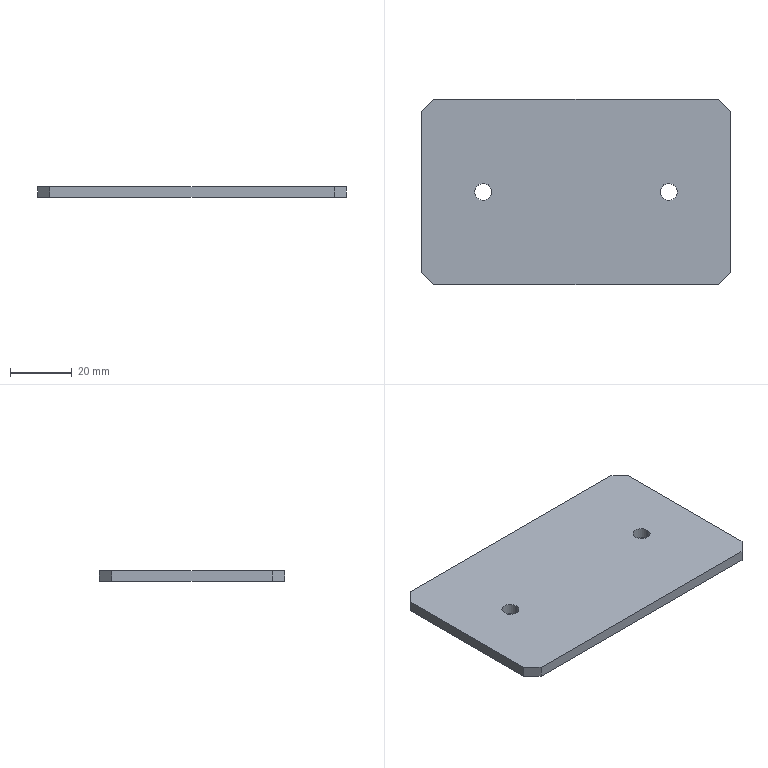Part | STEP file | B1-031 | 1 solid | 14 faces | box 100 x 60 x 3.5 mm | volume 20722 mm3 | plane 10 | cylinder 4 | commonest cylinder face diameters 5.5 x4
STEP:
#1=CARTESIAN_POINT('',(0.,0.,0.));
#2=DIRECTION('',(0.,0.,1.));
#3=DIRECTION('',(1.,0.,0.));
#4=AXIS2_PLACEMENT_3D('',#1,#2,#3);
#5=CARTESIAN_POINT('',(32.75,0.,-1.75));
#6=VERTEX_POINT('',#5);
#7=CARTESIAN_POINT('',(32.75,0.,1.75));
#8=VERTEX_POINT('',#7);
#9=CARTESIAN_POINT('',(32.75,0.,-9.528));
#10=DIRECTION('',(0.,0.,1.));
#11=VECTOR('',#10,1.);
#12=LINE('',#9,#11);
#13=CARTESIAN_POINT('',(30.,0.,-9.528));
#14=DIRECTION('',(0.,0.,1.));
#15=DIRECTION('',(1.,0.,0.));
#16=AXIS2_PLACEMENT_3D('',#13,#14,#15);
#17=CYLINDRICAL_SURFACE('',#16,2.75);
#18=CARTESIAN_POINT('',(6.283,0.));
#19=DIRECTION('',(0.,1.));
#20=VECTOR('',#19,1.);
#21=LINE('',#18,#20);
#22=(GEOMETRIC_REPRESENTATION_CONTEXT(2)PARAMETRIC_REPRESENTATION_CONTEXT()REPRESENTATION_CONTEXT('',''));
#23=DEFINITIONAL_REPRESENTATION('',(#21),#22);
#24=PCURVE('',#17,#23);
#25=CARTESIAN_POINT('',(30.,0.,-9.528));
#26=DIRECTION('',(0.,0.,1.));
#27=DIRECTION('',(1.,0.,0.));
#28=AXIS2_PLACEMENT_3D('',#25,#26,#27);
#29=CYLINDRICAL_SURFACE('',#28,2.75);
#30=CARTESIAN_POINT('',(0.,0.));
#31=DIRECTION('',(0.,1.));
#32=VECTOR('',#31,1.);
#33=LINE('',#30,#32);
#34=(GEOMETRIC_REPRESENTATION_CONTEXT(2)PARAMETRIC_REPRESENTATION_CONTEXT()REPRESENTATION_CONTEXT('',''));
#35=DEFINITIONAL_REPRESENTATION('',(#33),#34);
#36=PCURVE('',#29,#35);
#37=SURFACE_CURVE('',#12,(#24,#36),.PCURVE_S1.);
#38=EDGE_CURVE('',#6,#8,#37,.T.);
#39=ORIENTED_EDGE('',*,*,#38,.T.);
#40=CARTESIAN_POINT('',(27.25,0.,1.75));
#41=VERTEX_POINT('',#40);
#42=CARTESIAN_POINT('',(30.,0.,1.75));
#43=DIRECTION('',(0.,0.,1.));
#44=DIRECTION('',(1.,0.,0.));
#45=AXIS2_PLACEMENT_3D('',#42,#43,#44);
#46=CIRCLE('',#45,2.75);
#47=CARTESIAN_POINT('',(0.,11.278));
#48=DIRECTION('',(1.,0.));
#49=VECTOR('',#48,1.);
#50=LINE('',#47,#49);
#51=(GEOMETRIC_REPRESENTATION_CONTEXT(2)PARAMETRIC_REPRESENTATION_CONTEXT()REPRESENTATION_CONTEXT('',''));
#52=DEFINITIONAL_REPRESENTATION('',(#50),#51);
#53=PCURVE('',#17,#52);
#54=CARTESIAN_POINT('',(0.,0.,1.75));
#55=DIRECTION('',(0.,0.,1.));
#56=DIRECTION('',(1.,0.,0.));
#57=AXIS2_PLACEMENT_3D('',#54,#55,#56);
#58=PLANE('',#57);
#59=CARTESIAN_POINT('',(30.,0.));
#60=DIRECTION('',(1.,0.));
#61=AXIS2_PLACEMENT_2D('',#59,#60);
#62=CIRCLE('',#61,2.75);
#63=(GEOMETRIC_REPRESENTATION_CONTEXT(2)PARAMETRIC_REPRESENTATION_CONTEXT()REPRESENTATION_CONTEXT('',''));
#64=DEFINITIONAL_REPRESENTATION('',(#62),#63);
#65=PCURVE('',#58,#64);
#66=SURFACE_CURVE('',#46,(#53,#65),.PCURVE_S1.);
#67=EDGE_CURVE('',#41,#8,#66,.T.);
#68=ORIENTED_EDGE('',*,*,#67,.F.);
#69=CARTESIAN_POINT('',(27.25,0.,-1.75));
#70=VERTEX_POINT('',#69);
#71=CARTESIAN_POINT('',(27.25,0.,-9.528));
#72=DIRECTION('',(0.,0.,1.));
#73=VECTOR('',#72,1.);
#74=LINE('',#71,#73);
#75=CARTESIAN_POINT('',(3.142,0.));
#76=DIRECTION('',(0.,1.));
#77=VECTOR('',#76,1.);
#78=LINE('',#75,#77);
#79=(GEOMETRIC_REPRESENTATION_CONTEXT(2)PARAMETRIC_REPRESENTATION_CONTEXT()REPRESENTATION_CONTEXT('',''));
#80=DEFINITIONAL_REPRESENTATION('',(#78),#79);
#81=PCURVE('',#17,#80);
#82=CARTESIAN_POINT('',(3.142,0.));
#83=DIRECTION('',(0.,1.));
#84=VECTOR('',#83,1.);
#85=LINE('',#82,#84);
#86=(GEOMETRIC_REPRESENTATION_CONTEXT(2)PARAMETRIC_REPRESENTATION_CONTEXT()REPRESENTATION_CONTEXT('',''));
#87=DEFINITIONAL_REPRESENTATION('',(#85),#86);
#88=PCURVE('',#29,#87);
#89=SURFACE_CURVE('',#74,(#81,#88),.PCURVE_S1.);
#90=EDGE_CURVE('',#70,#41,#89,.T.);
#91=ORIENTED_EDGE('',*,*,#90,.F.);
#92=CARTESIAN_POINT('',(30.,0.,-1.75));
#93=DIRECTION('',(0.,0.,-1.));
#94=DIRECTION('',(1.,0.,0.));
#95=AXIS2_PLACEMENT_3D('',#92,#93,#94);
#96=CIRCLE('',#95,2.75);
#97=CARTESIAN_POINT('',(6.283,7.778));
#98=DIRECTION('',(-1.,0.));
#99=VECTOR('',#98,1.);
#100=LINE('',#97,#99);
#101=(GEOMETRIC_REPRESENTATION_CONTEXT(2)PARAMETRIC_REPRESENTATION_CONTEXT()REPRESENTATION_CONTEXT('',''));
#102=DEFINITIONAL_REPRESENTATION('',(#100),#101);
#103=PCURVE('',#17,#102);
#104=CARTESIAN_POINT('',(0.,0.,-1.75));
#105=DIRECTION('',(0.,0.,1.));
#106=DIRECTION('',(1.,0.,0.));
#107=AXIS2_PLACEMENT_3D('',#104,#105,#106);
#108=PLANE('',#107);
#109=CARTESIAN_POINT('',(32.75,0.));
#110=CARTESIAN_POINT('',(32.75,-4.763));
#111=CARTESIAN_POINT('',(28.625,-2.382));
#112=CARTESIAN_POINT('',(24.5,0.));
#113=CARTESIAN_POINT('',(28.625,2.382));
#114=CARTESIAN_POINT('',(32.75,4.763));
#115=CARTESIAN_POINT('',(32.75,0.));
#116=(BOUNDED_CURVE()B_SPLINE_CURVE(2,(#109,#110,#111,#112,#113,#114,#115),.UNSPECIFIED.,.T.,.F.)B_SPLINE_CURVE_WITH_KNOTS((1,2,2,2,2,1),(-2.094,0.,2.094,4.189,6.283,8.378),.UNSPECIFIED.)CURVE()GEOMETRIC_REPRESENTATION_ITEM()RATIONAL_B_SPLINE_CURVE((1.,0.5,1.,0.5,1.,0.5,1.))REPRESENTATION_ITEM(''));
#117=(GEOMETRIC_REPRESENTATION_CONTEXT(2)PARAMETRIC_REPRESENTATION_CONTEXT()REPRESENTATION_CONTEXT('',''));
#118=DEFINITIONAL_REPRESENTATION('',(#116),#117);
#119=PCURVE('',#108,#118);
#120=SURFACE_CURVE('',#96,(#103,#119),.PCURVE_S1.);
#121=EDGE_CURVE('',#6,#70,#120,.T.);
#122=ORIENTED_EDGE('',*,*,#121,.F.);
#123=EDGE_LOOP('',(#39,#68,#91,#122));
#124=FACE_BOUND('',#123,.F.);
#125=ADVANCED_FACE('',(#124),#17,.F.);
#126=CARTESIAN_POINT('',(-27.25,0.,-1.75));
#127=VERTEX_POINT('',#126);
#128=CARTESIAN_POINT('',(-27.25,0.,1.75));
#129=VERTEX_POINT('',#128);
#130=CARTESIAN_POINT('',(-27.25,0.,-9.528));
#131=DIRECTION('',(0.,0.,1.));
#132=VECTOR('',#131,1.);
#133=LINE('',#130,#132);
#134=CARTESIAN_POINT('',(-30.,0.,-9.528));
#135=DIRECTION('',(0.,0.,1.));
#136=DIRECTION('',(1.,0.,0.));
#137=AXIS2_PLACEMENT_3D('',#134,#135,#136);
#138=CYLINDRICAL_SURFACE('',#137,2.75);
#139=CARTESIAN_POINT('',(6.283,0.));
#140=DIRECTION('',(0.,1.));
#141=VECTOR('',#140,1.);
#142=LINE('',#139,#141);
#143=(GEOMETRIC_REPRESENTATION_CONTEXT(2)PARAMETRIC_REPRESENTATION_CONTEXT()REPRESENTATION_CONTEXT('',''));
#144=DEFINITIONAL_REPRESENTATION('',(#142),#143);
#145=PCURVE('',#138,#144);
#146=CARTESIAN_POINT('',(-30.,0.,-9.528));
#147=DIRECTION('',(0.,0.,1.));
#148=DIRECTION('',(1.,0.,0.));
#149=AXIS2_PLACEMENT_3D('',#146,#147,#148);
#150=CYLINDRICAL_SURFACE('',#149,2.75);
#151=CARTESIAN_POINT('',(0.,0.));
#152=DIRECTION('',(0.,1.));
#153=VECTOR('',#152,1.);
#154=LINE('',#151,#153);
#155=(GEOMETRIC_REPRESENTATION_CONTEXT(2)PARAMETRIC_REPRESENTATION_CONTEXT()REPRESENTATION_CONTEXT('',''));
#156=DEFINITIONAL_REPRESENTATION('',(#154),#155);
#157=PCURVE('',#150,#156);
#158=SURFACE_CURVE('',#133,(#145,#157),.PCURVE_S1.);
#159=EDGE_CURVE('',#127,#129,#158,.T.);
#160=ORIENTED_EDGE('',*,*,#159,.T.);
#161=CARTESIAN_POINT('',(-32.75,0.,1.75));
#162=VERTEX_POINT('',#161);
#163=CARTESIAN_POINT('',(-30.,0.,1.75));
#164=DIRECTION('',(0.,0.,1.));
#165=DIRECTION('',(1.,0.,0.));
#166=AXIS2_PLACEMENT_3D('',#163,#164,#165);
#167=CIRCLE('',#166,2.75);
#168=CARTESIAN_POINT('',(0.,11.278));
#169=DIRECTION('',(1.,0.));
#170=VECTOR('',#169,1.);
#171=LINE('',#168,#170);
#172=(GEOMETRIC_REPRESENTATION_CONTEXT(2)PARAMETRIC_REPRESENTATION_CONTEXT()REPRESENTATION_CONTEXT('',''));
#173=DEFINITIONAL_REPRESENTATION('',(#171),#172);
#174=PCURVE('',#138,#173);
#175=CARTESIAN_POINT('',(-30.,0.));
#176=DIRECTION('',(1.,0.));
#177=AXIS2_PLACEMENT_2D('',#175,#176);
#178=CIRCLE('',#177,2.75);
#179=(GEOMETRIC_REPRESENTATION_CONTEXT(2)PARAMETRIC_REPRESENTATION_CONTEXT()REPRESENTATION_CONTEXT('',''));
#180=DEFINITIONAL_REPRESENTATION('',(#178),#179);
#181=PCURVE('',#58,#180);
#182=SURFACE_CURVE('',#167,(#174,#181),.PCURVE_S1.);
#183=EDGE_CURVE('',#162,#129,#182,.T.);
#184=ORIENTED_EDGE('',*,*,#183,.F.);
#185=CARTESIAN_POINT('',(-32.75,0.,-1.75));
#186=VERTEX_POINT('',#185);
#187=CARTESIAN_POINT('',(-32.75,0.,-9.528));
#188=DIRECTION('',(0.,0.,1.));
#189=VECTOR('',#188,1.);
#190=LINE('',#187,#189);
#191=CARTESIAN_POINT('',(3.142,0.));
#192=DIRECTION('',(0.,1.));
#193=VECTOR('',#192,1.);
#194=LINE('',#191,#193);
#195=(GEOMETRIC_REPRESENTATION_CONTEXT(2)PARAMETRIC_REPRESENTATION_CONTEXT()REPRESENTATION_CONTEXT('',''));
#196=DEFINITIONAL_REPRESENTATION('',(#194),#195);
#197=PCURVE('',#138,#196);
#198=CARTESIAN_POINT('',(3.142,0.));
#199=DIRECTION('',(0.,1.));
#200=VECTOR('',#199,1.);
#201=LINE('',#198,#200);
#202=(GEOMETRIC_REPRESENTATION_CONTEXT(2)PARAMETRIC_REPRESENTATION_CONTEXT()REPRESENTATION_CONTEXT('',''));
#203=DEFINITIONAL_REPRESENTATION('',(#201),#202);
#204=PCURVE('',#150,#203);
#205=SURFACE_CURVE('',#190,(#197,#204),.PCURVE_S1.);
#206=EDGE_CURVE('',#186,#162,#205,.T.);
#207=ORIENTED_EDGE('',*,*,#206,.F.);
#208=CARTESIAN_POINT('',(-30.,0.,-1.75));
#209=DIRECTION('',(0.,0.,-1.));
#210=DIRECTION('',(1.,0.,0.));
#211=AXIS2_PLACEMENT_3D('',#208,#209,#210);
#212=CIRCLE('',#211,2.75);
#213=CARTESIAN_POINT('',(6.283,7.778));
#214=DIRECTION('',(-1.,0.));
#215=VECTOR('',#214,1.);
#216=LINE('',#213,#215);
#217=(GEOMETRIC_REPRESENTATION_CONTEXT(2)PARAMETRIC_REPRESENTATION_CONTEXT()REPRESENTATION_CONTEXT('',''));
#218=DEFINITIONAL_REPRESENTATION('',(#216),#217);
#219=PCURVE('',#138,#218);
#220=CARTESIAN_POINT('',(-27.25,0.));
#221=CARTESIAN_POINT('',(-27.25,-4.763));
#222=CARTESIAN_POINT('',(-31.375,-2.382));
#223=CARTESIAN_POINT('',(-35.5,0.));
#224=CARTESIAN_POINT('',(-31.375,2.382));
#225=CARTESIAN_POINT('',(-27.25,4.763));
#226=CARTESIAN_POINT('',(-27.25,0.));
#227=(BOUNDED_CURVE()B_SPLINE_CURVE(2,(#220,#221,#222,#223,#224,#225,#226),.UNSPECIFIED.,.T.,.F.)B_SPLINE_CURVE_WITH_KNOTS((1,2,2,2,2,1),(-2.094,0.,2.094,4.189,6.283,8.378),.UNSPECIFIED.)CURVE()GEOMETRIC_REPRESENTATION_ITEM()RATIONAL_B_SPLINE_CURVE((1.,0.5,1.,0.5,1.,0.5,1.))REPRESENTATION_ITEM(''));
#228=(GEOMETRIC_REPRESENTATION_CONTEXT(2)PARAMETRIC_REPRESENTATION_CONTEXT()REPRESENTATION_CONTEXT('',''));
#229=DEFINITIONAL_REPRESENTATION('',(#227),#228);
#230=PCURVE('',#108,#229);
#231=SURFACE_CURVE('',#212,(#219,#230),.PCURVE_S1.);
#232=EDGE_CURVE('',#127,#186,#231,.T.);
#233=ORIENTED_EDGE('',*,*,#232,.F.);
#234=EDGE_LOOP('',(#160,#184,#207,#233));
#235=FACE_BOUND('',#234,.F.);
#236=ADVANCED_FACE('',(#235),#138,.F.);
#237=CARTESIAN_POINT('',(50.,-26.,1.75));
#238=VERTEX_POINT('',#237);
#239=CARTESIAN_POINT('',(50.,26.,1.75));
#240=VERTEX_POINT('',#239);
#241=CARTESIAN_POINT('',(50.,30.,1.75));
#242=DIRECTION('',(0.,1.,0.));
#243=VECTOR('',#242,1.);
#244=LINE('',#241,#243);
#245=CARTESIAN_POINT('',(50.,30.,1.75));
#246=DIRECTION('',(-1.,0.,0.));
#247=DIRECTION('',(0.,0.,1.));
#248=AXIS2_PLACEMENT_3D('',#245,#246,#247);
#249=PLANE('',#248);
#250=CARTESIAN_POINT('',(0.,0.));
#251=DIRECTION('',(0.,1.));
#252=VECTOR('',#251,1.);
#253=LINE('',#250,#252);
#254=(GEOMETRIC_REPRESENTATION_CONTEXT(2)PARAMETRIC_REPRESENTATION_CONTEXT()REPRESENTATION_CONTEXT('',''));
#255=DEFINITIONAL_REPRESENTATION('',(#253),#254);
#256=PCURVE('',#249,#255);
#257=CARTESIAN_POINT('',(50.,30.));
#258=DIRECTION('',(0.,1.));
#259=VECTOR('',#258,1.);
#260=LINE('',#257,#259);
#261=(GEOMETRIC_REPRESENTATION_CONTEXT(2)PARAMETRIC_REPRESENTATION_CONTEXT()REPRESENTATION_CONTEXT('',''));
#262=DEFINITIONAL_REPRESENTATION('',(#260),#261);
#263=PCURVE('',#58,#262);
#264=SURFACE_CURVE('',#244,(#256,#263),.PCURVE_S1.);
#265=EDGE_CURVE('',#238,#240,#264,.T.);
#266=ORIENTED_EDGE('',*,*,#265,.F.);
#267=CARTESIAN_POINT('',(50.,-26.,-1.75));
#268=VERTEX_POINT('',#267);
#269=CARTESIAN_POINT('',(50.,-26.,1.75));
#270=DIRECTION('',(0.,0.,-1.));
#271=VECTOR('',#270,1.);
#272=LINE('',#269,#271);
#273=CARTESIAN_POINT('',(0.,-56.));
#274=DIRECTION('',(-1.,0.));
#275=VECTOR('',#274,1.);
#276=LINE('',#273,#275);
#277=(GEOMETRIC_REPRESENTATION_CONTEXT(2)PARAMETRIC_REPRESENTATION_CONTEXT()REPRESENTATION_CONTEXT('',''));
#278=DEFINITIONAL_REPRESENTATION('',(#276),#277);
#279=PCURVE('',#249,#278);
#280=CARTESIAN_POINT('',(50.,-26.,1.75));
#281=DIRECTION('',(-0.7071,0.7071,0.));
#282=DIRECTION('',(0.,0.,-1.));
#283=AXIS2_PLACEMENT_3D('',#280,#281,#282);
#284=PLANE('',#283);
#285=CARTESIAN_POINT('',(0.,0.));
#286=DIRECTION('',(1.,0.));
#287=VECTOR('',#286,1.);
#288=LINE('',#285,#287);
#289=(GEOMETRIC_REPRESENTATION_CONTEXT(2)PARAMETRIC_REPRESENTATION_CONTEXT()REPRESENTATION_CONTEXT('',''));
#290=DEFINITIONAL_REPRESENTATION('',(#288),#289);
#291=PCURVE('',#284,#290);
#292=SURFACE_CURVE('',#272,(#279,#291),.PCURVE_S1.);
#293=EDGE_CURVE('',#238,#268,#292,.T.);
#294=ORIENTED_EDGE('',*,*,#293,.T.);
#295=CARTESIAN_POINT('',(50.,26.,-1.75));
#296=VERTEX_POINT('',#295);
#297=CARTESIAN_POINT('',(50.,30.,-1.75));
#298=DIRECTION('',(0.,1.,0.));
#299=VECTOR('',#298,1.);
#300=LINE('',#297,#299);
#301=CARTESIAN_POINT('',(-3.5,0.));
#302=DIRECTION('',(0.,1.));
#303=VECTOR('',#302,1.);
#304=LINE('',#301,#303);
#305=(GEOMETRIC_REPRESENTATION_CONTEXT(2)PARAMETRIC_REPRESENTATION_CONTEXT()REPRESENTATION_CONTEXT('',''));
#306=DEFINITIONAL_REPRESENTATION('',(#304),#305);
#307=PCURVE('',#249,#306);
#308=CARTESIAN_POINT('',(50.,30.));
#309=DIRECTION('',(0.,1.));
#310=VECTOR('',#309,1.);
#311=LINE('',#308,#310);
#312=(GEOMETRIC_REPRESENTATION_CONTEXT(2)PARAMETRIC_REPRESENTATION_CONTEXT()REPRESENTATION_CONTEXT('',''));
#313=DEFINITIONAL_REPRESENTATION('',(#311),#312);
#314=PCURVE('',#108,#313);
#315=SURFACE_CURVE('',#300,(#307,#314),.PCURVE_S1.);
#316=EDGE_CURVE('',#268,#296,#315,.T.);
#317=ORIENTED_EDGE('',*,*,#316,.T.);
#318=CARTESIAN_POINT('',(50.,26.,1.75));
#319=DIRECTION('',(0.,0.,1.));
#320=VECTOR('',#319,1.);
#321=LINE('',#318,#320);
#322=CARTESIAN_POINT('',(0.,-4.));
#323=DIRECTION('',(1.,0.));
#324=VECTOR('',#323,1.);
#325=LINE('',#322,#324);
#326=(GEOMETRIC_REPRESENTATION_CONTEXT(2)PARAMETRIC_REPRESENTATION_CONTEXT()REPRESENTATION_CONTEXT('',''));
#327=DEFINITIONAL_REPRESENTATION('',(#325),#326);
#328=PCURVE('',#249,#327);
#329=CARTESIAN_POINT('',(46.,30.,1.75));
#330=DIRECTION('',(-0.7071,-0.7071,0.));
#331=DIRECTION('',(0.,0.,-1.));
#332=AXIS2_PLACEMENT_3D('',#329,#330,#331);
#333=PLANE('',#332);
#334=CARTESIAN_POINT('',(0.,5.657));
#335=DIRECTION('',(-1.,0.));
#336=VECTOR('',#335,1.);
#337=LINE('',#334,#336);
#338=(GEOMETRIC_REPRESENTATION_CONTEXT(2)PARAMETRIC_REPRESENTATION_CONTEXT()REPRESENTATION_CONTEXT('',''));
#339=DEFINITIONAL_REPRESENTATION('',(#337),#338);
#340=PCURVE('',#333,#339);
#341=SURFACE_CURVE('',#321,(#328,#340),.PCURVE_S1.);
#342=EDGE_CURVE('',#296,#240,#341,.T.);
#343=ORIENTED_EDGE('',*,*,#342,.T.);
#344=EDGE_LOOP('',(#266,#294,#317,#343));
#345=FACE_BOUND('',#344,.T.);
#346=ADVANCED_FACE('',(#345),#249,.F.);
#347=CARTESIAN_POINT('',(46.,30.,-1.75));
#348=VERTEX_POINT('',#347);
#349=CARTESIAN_POINT('',(-46.,30.,-1.75));
#350=VERTEX_POINT('',#349);
#351=CARTESIAN_POINT('',(-50.,30.,-1.75));
#352=DIRECTION('',(-1.,0.,0.));
#353=VECTOR('',#352,1.);
#354=LINE('',#351,#353);
#355=CARTESIAN_POINT('',(-50.,30.,1.75));
#356=DIRECTION('',(0.,-1.,0.));
#357=DIRECTION('',(0.,0.,-1.));
#358=AXIS2_PLACEMENT_3D('',#355,#356,#357);
#359=PLANE('',#358);
#360=CARTESIAN_POINT('',(3.5,0.));
#361=DIRECTION('',(0.,-1.));
#362=VECTOR('',#361,1.);
#363=LINE('',#360,#362);
#364=(GEOMETRIC_REPRESENTATION_CONTEXT(2)PARAMETRIC_REPRESENTATION_CONTEXT()REPRESENTATION_CONTEXT('',''));
#365=DEFINITIONAL_REPRESENTATION('',(#363),#364);
#366=PCURVE('',#359,#365);
#367=CARTESIAN_POINT('',(-50.,30.));
#368=DIRECTION('',(-1.,0.));
#369=VECTOR('',#368,1.);
#370=LINE('',#367,#369);
#371=(GEOMETRIC_REPRESENTATION_CONTEXT(2)PARAMETRIC_REPRESENTATION_CONTEXT()REPRESENTATION_CONTEXT('',''));
#372=DEFINITIONAL_REPRESENTATION('',(#370),#371);
#373=PCURVE('',#108,#372);
#374=SURFACE_CURVE('',#354,(#366,#373),.PCURVE_S1.);
#375=EDGE_CURVE('',#348,#350,#374,.T.);
#376=ORIENTED_EDGE('',*,*,#375,.T.);
#377=CARTESIAN_POINT('',(-46.,30.,1.75));
#378=VERTEX_POINT('',#377);
#379=CARTESIAN_POINT('',(-46.,30.,1.75));
#380=DIRECTION('',(0.,0.,1.));
#381=VECTOR('',#380,1.);
#382=LINE('',#379,#381);
#383=CARTESIAN_POINT('',(0.,4.));
#384=DIRECTION('',(-1.,0.));
#385=VECTOR('',#384,1.);
#386=LINE('',#383,#385);
#387=(GEOMETRIC_REPRESENTATION_CONTEXT(2)PARAMETRIC_REPRESENTATION_CONTEXT()REPRESENTATION_CONTEXT('',''));
#388=DEFINITIONAL_REPRESENTATION('',(#386),#387);
#389=PCURVE('',#359,#388);
#390=CARTESIAN_POINT('',(-50.,26.,1.75));
#391=DIRECTION('',(0.7071,-0.7071,0.));
#392=DIRECTION('',(0.,0.,-1.));
#393=AXIS2_PLACEMENT_3D('',#390,#391,#392);
#394=PLANE('',#393);
#395=CARTESIAN_POINT('',(0.,5.657));
#396=DIRECTION('',(-1.,0.));
#397=VECTOR('',#396,1.);
#398=LINE('',#395,#397);
#399=(GEOMETRIC_REPRESENTATION_CONTEXT(2)PARAMETRIC_REPRESENTATION_CONTEXT()REPRESENTATION_CONTEXT('',''));
#400=DEFINITIONAL_REPRESENTATION('',(#398),#399);
#401=PCURVE('',#394,#400);
#402=SURFACE_CURVE('',#382,(#389,#401),.PCURVE_S1.);
#403=EDGE_CURVE('',#350,#378,#402,.T.);
#404=ORIENTED_EDGE('',*,*,#403,.T.);
#405=CARTESIAN_POINT('',(46.,30.,1.75));
#406=VERTEX_POINT('',#405);
#407=CARTESIAN_POINT('',(-50.,30.,1.75));
#408=DIRECTION('',(-1.,0.,0.));
#409=VECTOR('',#408,1.);
#410=LINE('',#407,#409);
#411=CARTESIAN_POINT('',(0.,0.));
#412=DIRECTION('',(0.,-1.));
#413=VECTOR('',#412,1.);
#414=LINE('',#411,#413);
#415=(GEOMETRIC_REPRESENTATION_CONTEXT(2)PARAMETRIC_REPRESENTATION_CONTEXT()REPRESENTATION_CONTEXT('',''));
#416=DEFINITIONAL_REPRESENTATION('',(#414),#415);
#417=PCURVE('',#359,#416);
#418=CARTESIAN_POINT('',(-50.,30.));
#419=DIRECTION('',(-1.,0.));
#420=VECTOR('',#419,1.);
#421=LINE('',#418,#420);
#422=(GEOMETRIC_REPRESENTATION_CONTEXT(2)PARAMETRIC_REPRESENTATION_CONTEXT()REPRESENTATION_CONTEXT('',''));
#423=DEFINITIONAL_REPRESENTATION('',(#421),#422);
#424=PCURVE('',#58,#423);
#425=SURFACE_CURVE('',#410,(#417,#424),.PCURVE_S1.);
#426=EDGE_CURVE('',#406,#378,#425,.T.);
#427=ORIENTED_EDGE('',*,*,#426,.F.);
#428=CARTESIAN_POINT('',(46.,30.,1.75));
#429=DIRECTION('',(0.,0.,-1.));
#430=VECTOR('',#429,1.);
#431=LINE('',#428,#430);
#432=CARTESIAN_POINT('',(0.,96.));
#433=DIRECTION('',(1.,0.));
#434=VECTOR('',#433,1.);
#435=LINE('',#432,#434);
#436=(GEOMETRIC_REPRESENTATION_CONTEXT(2)PARAMETRIC_REPRESENTATION_CONTEXT()REPRESENTATION_CONTEXT('',''));
#437=DEFINITIONAL_REPRESENTATION('',(#435),#436);
#438=PCURVE('',#359,#437);
#439=CARTESIAN_POINT('',(0.,0.));
#440=DIRECTION('',(1.,0.));
#441=VECTOR('',#440,1.);
#442=LINE('',#439,#441);
#443=(GEOMETRIC_REPRESENTATION_CONTEXT(2)PARAMETRIC_REPRESENTATION_CONTEXT()REPRESENTATION_CONTEXT('',''));
#444=DEFINITIONAL_REPRESENTATION('',(#442),#443);
#445=PCURVE('',#333,#444);
#446=SURFACE_CURVE('',#431,(#438,#445),.PCURVE_S1.);
#447=EDGE_CURVE('',#406,#348,#446,.T.);
#448=ORIENTED_EDGE('',*,*,#447,.T.);
#449=EDGE_LOOP('',(#376,#404,#427,#448));
#450=FACE_BOUND('',#449,.T.);
#451=ADVANCED_FACE('',(#450),#359,.F.);
#452=CARTESIAN_POINT('',(-50.,26.,1.75));
#453=VERTEX_POINT('',#452);
#454=CARTESIAN_POINT('',(-50.,-26.,1.75));
#455=VERTEX_POINT('',#454);
#456=CARTESIAN_POINT('',(-50.,30.,1.75));
#457=DIRECTION('',(0.,-1.,0.));
#458=VECTOR('',#457,1.);
#459=LINE('',#456,#458);
#460=CARTESIAN_POINT('',(-50.,30.,1.75));
#461=DIRECTION('',(1.,0.,0.));
#462=DIRECTION('',(0.,0.,-1.));
#463=AXIS2_PLACEMENT_3D('',#460,#461,#462);
#464=PLANE('',#463);
#465=CARTESIAN_POINT('',(0.,0.));
#466=DIRECTION('',(0.,-1.));
#467=VECTOR('',#466,1.);
#468=LINE('',#465,#467);
#469=(GEOMETRIC_REPRESENTATION_CONTEXT(2)PARAMETRIC_REPRESENTATION_CONTEXT()REPRESENTATION_CONTEXT('',''));
#470=DEFINITIONAL_REPRESENTATION('',(#468),#469);
#471=PCURVE('',#464,#470);
#472=CARTESIAN_POINT('',(-50.,30.));
#473=DIRECTION('',(0.,-1.));
#474=VECTOR('',#473,1.);
#475=LINE('',#472,#474);
#476=(GEOMETRIC_REPRESENTATION_CONTEXT(2)PARAMETRIC_REPRESENTATION_CONTEXT()REPRESENTATION_CONTEXT('',''));
#477=DEFINITIONAL_REPRESENTATION('',(#475),#476);
#478=PCURVE('',#58,#477);
#479=SURFACE_CURVE('',#459,(#471,#478),.PCURVE_S1.);
#480=EDGE_CURVE('',#453,#455,#479,.T.);
#481=ORIENTED_EDGE('',*,*,#480,.F.);
#482=CARTESIAN_POINT('',(-50.,26.,-1.75));
#483=VERTEX_POINT('',#482);
#484=CARTESIAN_POINT('',(-50.,26.,1.75));
#485=DIRECTION('',(0.,0.,-1.));
#486=VECTOR('',#485,1.);
#487=LINE('',#484,#486);
#488=CARTESIAN_POINT('',(0.,-4.));
#489=DIRECTION('',(1.,0.));
#490=VECTOR('',#489,1.);
#491=LINE('',#488,#490);
#492=(GEOMETRIC_REPRESENTATION_CONTEXT(2)PARAMETRIC_REPRESENTATION_CONTEXT()REPRESENTATION_CONTEXT('',''));
#493=DEFINITIONAL_REPRESENTATION('',(#491),#492);
#494=PCURVE('',#464,#493);
#495=CARTESIAN_POINT('',(0.,0.));
#496=DIRECTION('',(1.,0.));
#497=VECTOR('',#496,1.);
#498=LINE('',#495,#497);
#499=(GEOMETRIC_REPRESENTATION_CONTEXT(2)PARAMETRIC_REPRESENTATION_CONTEXT()REPRESENTATION_CONTEXT('',''));
#500=DEFINITIONAL_REPRESENTATION('',(#498),#499);
#501=PCURVE('',#394,#500);
#502=SURFACE_CURVE('',#487,(#494,#501),.PCURVE_S1.);
#503=EDGE_CURVE('',#453,#483,#502,.T.);
#504=ORIENTED_EDGE('',*,*,#503,.T.);
#505=CARTESIAN_POINT('',(-50.,-26.,-1.75));
#506=VERTEX_POINT('',#505);
#507=CARTESIAN_POINT('',(-50.,30.,-1.75));
#508=DIRECTION('',(0.,-1.,0.));
#509=VECTOR('',#508,1.);
#510=LINE('',#507,#509);
#511=CARTESIAN_POINT('',(3.5,0.));
#512=DIRECTION('',(0.,-1.));
#513=VECTOR('',#512,1.);
#514=LINE('',#511,#513);
#515=(GEOMETRIC_REPRESENTATION_CONTEXT(2)PARAMETRIC_REPRESENTATION_CONTEXT()REPRESENTATION_CONTEXT('',''));
#516=DEFINITIONAL_REPRESENTATION('',(#514),#515);
#517=PCURVE('',#464,#516);
#518=CARTESIAN_POINT('',(-50.,30.));
#519=DIRECTION('',(0.,-1.));
#520=VECTOR('',#519,1.);
#521=LINE('',#518,#520);
#522=(GEOMETRIC_REPRESENTATION_CONTEXT(2)PARAMETRIC_REPRESENTATION_CONTEXT()REPRESENTATION_CONTEXT('',''));
#523=DEFINITIONAL_REPRESENTATION('',(#521),#522);
#524=PCURVE('',#108,#523);
#525=SURFACE_CURVE('',#510,(#517,#524),.PCURVE_S1.);
#526=EDGE_CURVE('',#483,#506,#525,.T.);
#527=ORIENTED_EDGE('',*,*,#526,.T.);
#528=CARTESIAN_POINT('',(-50.,-26.,1.75));
#529=DIRECTION('',(0.,0.,1.));
#530=VECTOR('',#529,1.);
#531=LINE('',#528,#530);
#532=CARTESIAN_POINT('',(0.,-56.));
#533=DIRECTION('',(-1.,0.));
#534=VECTOR('',#533,1.);
#535=LINE('',#532,#534);
#536=(GEOMETRIC_REPRESENTATION_CONTEXT(2)PARAMETRIC_REPRESENTATION_CONTEXT()REPRESENTATION_CONTEXT('',''));
#537=DEFINITIONAL_REPRESENTATION('',(#535),#536);
#538=PCURVE('',#464,#537);
#539=CARTESIAN_POINT('',(-46.,-30.,1.75));
#540=DIRECTION('',(0.7071,0.7071,0.));
#541=DIRECTION('',(0.,0.,-1.));
#542=AXIS2_PLACEMENT_3D('',#539,#540,#541);
#543=PLANE('',#542);
#544=CARTESIAN_POINT('',(0.,5.657));
#545=DIRECTION('',(-1.,0.));
#546=VECTOR('',#545,1.);
#547=LINE('',#544,#546);
#548=(GEOMETRIC_REPRESENTATION_CONTEXT(2)PARAMETRIC_REPRESENTATION_CONTEXT()REPRESENTATION_CONTEXT('',''));
#549=DEFINITIONAL_REPRESENTATION('',(#547),#548);
#550=PCURVE('',#543,#549);
#551=SURFACE_CURVE('',#531,(#538,#550),.PCURVE_S1.);
#552=EDGE_CURVE('',#506,#455,#551,.T.);
#553=ORIENTED_EDGE('',*,*,#552,.T.);
#554=EDGE_LOOP('',(#481,#504,#527,#553));
#555=FACE_BOUND('',#554,.T.);
#556=ADVANCED_FACE('',(#555),#464,.F.);
#557=CARTESIAN_POINT('',(-46.,-30.,1.75));
#558=VERTEX_POINT('',#557);
#559=CARTESIAN_POINT('',(46.,-30.,1.75));
#560=VERTEX_POINT('',#559);
#561=CARTESIAN_POINT('',(-50.,-30.,1.75));
#562=DIRECTION('',(1.,0.,0.));
#563=VECTOR('',#562,1.);
#564=LINE('',#561,#563);
#565=CARTESIAN_POINT('',(-50.,-30.,1.75));
#566=DIRECTION('',(0.,1.,0.));
#567=DIRECTION('',(0.,0.,1.));
#568=AXIS2_PLACEMENT_3D('',#565,#566,#567);
#569=PLANE('',#568);
#570=CARTESIAN_POINT('',(0.,0.));
#571=DIRECTION('',(0.,1.));
#572=VECTOR('',#571,1.);
#573=LINE('',#570,#572);
#574=(GEOMETRIC_REPRESENTATION_CONTEXT(2)PARAMETRIC_REPRESENTATION_CONTEXT()REPRESENTATION_CONTEXT('',''));
#575=DEFINITIONAL_REPRESENTATION('',(#573),#574);
#576=PCURVE('',#569,#575);
#577=CARTESIAN_POINT('',(-50.,-30.));
#578=DIRECTION('',(1.,0.));
#579=VECTOR('',#578,1.);
#580=LINE('',#577,#579);
#581=(GEOMETRIC_REPRESENTATION_CONTEXT(2)PARAMETRIC_REPRESENTATION_CONTEXT()REPRESENTATION_CONTEXT('',''));
#582=DEFINITIONAL_REPRESENTATION('',(#580),#581);
#583=PCURVE('',#58,#582);
#584=SURFACE_CURVE('',#564,(#576,#583),.PCURVE_S1.);
#585=EDGE_CURVE('',#558,#560,#584,.T.);
#586=ORIENTED_EDGE('',*,*,#585,.F.);
#587=CARTESIAN_POINT('',(-46.,-30.,-1.75));
#588=VERTEX_POINT('',#587);
#589=CARTESIAN_POINT('',(-46.,-30.,1.75));
#590=DIRECTION('',(0.,0.,-1.));
#591=VECTOR('',#590,1.);
#592=LINE('',#589,#591);
#593=CARTESIAN_POINT('',(0.,4.));
#594=DIRECTION('',(-1.,0.));
#595=VECTOR('',#594,1.);
#596=LINE('',#593,#595);
#597=(GEOMETRIC_REPRESENTATION_CONTEXT(2)PARAMETRIC_REPRESENTATION_CONTEXT()REPRESENTATION_CONTEXT('',''));
#598=DEFINITIONAL_REPRESENTATION('',(#596),#597);
#599=PCURVE('',#569,#598);
#600=CARTESIAN_POINT('',(0.,0.));
#601=DIRECTION('',(1.,0.));
#602=VECTOR('',#601,1.);
#603=LINE('',#600,#602);
#604=(GEOMETRIC_REPRESENTATION_CONTEXT(2)PARAMETRIC_REPRESENTATION_CONTEXT()REPRESENTATION_CONTEXT('',''));
#605=DEFINITIONAL_REPRESENTATION('',(#603),#604);
#606=PCURVE('',#543,#605);
#607=SURFACE_CURVE('',#592,(#599,#606),.PCURVE_S1.);
#608=EDGE_CURVE('',#558,#588,#607,.T.);
#609=ORIENTED_EDGE('',*,*,#608,.T.);
#610=CARTESIAN_POINT('',(46.,-30.,-1.75));
#611=VERTEX_POINT('',#610);
#612=CARTESIAN_POINT('',(-50.,-30.,-1.75));
#613=DIRECTION('',(1.,0.,0.));
#614=VECTOR('',#613,1.);
#615=LINE('',#612,#614);
#616=CARTESIAN_POINT('',(-3.5,0.));
#617=DIRECTION('',(0.,1.));
#618=VECTOR('',#617,1.);
#619=LINE('',#616,#618);
#620=(GEOMETRIC_REPRESENTATION_CONTEXT(2)PARAMETRIC_REPRESENTATION_CONTEXT()REPRESENTATION_CONTEXT('',''));
#621=DEFINITIONAL_REPRESENTATION('',(#619),#620);
#622=PCURVE('',#569,#621);
#623=CARTESIAN_POINT('',(-50.,-30.));
#624=DIRECTION('',(1.,0.));
#625=VECTOR('',#624,1.);
#626=LINE('',#623,#625);
#627=(GEOMETRIC_REPRESENTATION_CONTEXT(2)PARAMETRIC_REPRESENTATION_CONTEXT()REPRESENTATION_CONTEXT('',''));
#628=DEFINITIONAL_REPRESENTATION('',(#626),#627);
#629=PCURVE('',#108,#628);
#630=SURFACE_CURVE('',#615,(#622,#629),.PCURVE_S1.);
#631=EDGE_CURVE('',#588,#611,#630,.T.);
#632=ORIENTED_EDGE('',*,*,#631,.T.);
#633=CARTESIAN_POINT('',(46.,-30.,1.75));
#634=DIRECTION('',(0.,0.,1.));
#635=VECTOR('',#634,1.);
#636=LINE('',#633,#635);
#637=CARTESIAN_POINT('',(0.,96.));
#638=DIRECTION('',(1.,0.));
#639=VECTOR('',#638,1.);
#640=LINE('',#637,#639);
#641=(GEOMETRIC_REPRESENTATION_CONTEXT(2)PARAMETRIC_REPRESENTATION_CONTEXT()REPRESENTATION_CONTEXT('',''));
#642=DEFINITIONAL_REPRESENTATION('',(#640),#641);
#643=PCURVE('',#569,#642);
#644=CARTESIAN_POINT('',(0.,5.657));
#645=DIRECTION('',(-1.,0.));
#646=VECTOR('',#645,1.);
#647=LINE('',#644,#646);
#648=(GEOMETRIC_REPRESENTATION_CONTEXT(2)PARAMETRIC_REPRESENTATION_CONTEXT()REPRESENTATION_CONTEXT('',''));
#649=DEFINITIONAL_REPRESENTATION('',(#647),#648);
#650=PCURVE('',#284,#649);
#651=SURFACE_CURVE('',#636,(#643,#650),.PCURVE_S1.);
#652=EDGE_CURVE('',#611,#560,#651,.T.);
#653=ORIENTED_EDGE('',*,*,#652,.T.);
#654=EDGE_LOOP('',(#586,#609,#632,#653));
#655=FACE_BOUND('',#654,.T.);
#656=ADVANCED_FACE('',(#655),#569,.F.);
#657=CARTESIAN_POINT('',(30.,0.,1.75));
#658=DIRECTION('',(0.,0.,1.));
#659=DIRECTION('',(1.,0.,0.));
#660=AXIS2_PLACEMENT_3D('',#657,#658,#659);
#661=CIRCLE('',#660,2.75);
#662=CARTESIAN_POINT('',(30.,0.));
#663=DIRECTION('',(1.,0.));
#664=AXIS2_PLACEMENT_2D('',#662,#663);
#665=CIRCLE('',#664,2.75);
#666=(GEOMETRIC_REPRESENTATION_CONTEXT(2)PARAMETRIC_REPRESENTATION_CONTEXT()REPRESENTATION_CONTEXT('',''));
#667=DEFINITIONAL_REPRESENTATION('',(#665),#666);
#668=PCURVE('',#58,#667);
#669=CARTESIAN_POINT('',(0.,11.278));
#670=DIRECTION('',(1.,0.));
#671=VECTOR('',#670,1.);
#672=LINE('',#669,#671);
#673=(GEOMETRIC_REPRESENTATION_CONTEXT(2)PARAMETRIC_REPRESENTATION_CONTEXT()REPRESENTATION_CONTEXT('',''));
#674=DEFINITIONAL_REPRESENTATION('',(#672),#673);
#675=PCURVE('',#29,#674);
#676=SURFACE_CURVE('',#661,(#668,#675),.PCURVE_S1.);
#677=EDGE_CURVE('',#8,#41,#676,.T.);
#678=ORIENTED_EDGE('',*,*,#677,.F.);
#679=ORIENTED_EDGE('',*,*,#67,.F.);
#680=EDGE_LOOP('',(#678,#679));
#681=FACE_BOUND('',#680,.T.);
#682=CARTESIAN_POINT('',(-30.,0.,1.75));
#683=DIRECTION('',(0.,0.,1.));
#684=DIRECTION('',(1.,0.,0.));
#685=AXIS2_PLACEMENT_3D('',#682,#683,#684);
#686=CIRCLE('',#685,2.75);
#687=CARTESIAN_POINT('',(-30.,0.));
#688=DIRECTION('',(1.,0.));
#689=AXIS2_PLACEMENT_2D('',#687,#688);
#690=CIRCLE('',#689,2.75);
#691=(GEOMETRIC_REPRESENTATION_CONTEXT(2)PARAMETRIC_REPRESENTATION_CONTEXT()REPRESENTATION_CONTEXT('',''));
#692=DEFINITIONAL_REPRESENTATION('',(#690),#691);
#693=PCURVE('',#58,#692);
#694=CARTESIAN_POINT('',(0.,11.278));
#695=DIRECTION('',(1.,0.));
#696=VECTOR('',#695,1.);
#697=LINE('',#694,#696);
#698=(GEOMETRIC_REPRESENTATION_CONTEXT(2)PARAMETRIC_REPRESENTATION_CONTEXT()REPRESENTATION_CONTEXT('',''));
#699=DEFINITIONAL_REPRESENTATION('',(#697),#698);
#700=PCURVE('',#150,#699);
#701=SURFACE_CURVE('',#686,(#693,#700),.PCURVE_S1.);
#702=EDGE_CURVE('',#129,#162,#701,.T.);
#703=ORIENTED_EDGE('',*,*,#702,.F.);
#704=ORIENTED_EDGE('',*,*,#183,.F.);
#705=EDGE_LOOP('',(#703,#704));
#706=FACE_BOUND('',#705,.T.);
#707=ORIENTED_EDGE('',*,*,#426,.T.);
#708=CARTESIAN_POINT('',(-38.,38.,1.75));
#709=DIRECTION('',(-0.7071,-0.7071,0.));
#710=VECTOR('',#709,1.);
#711=LINE('',#708,#710);
#712=CARTESIAN_POINT('',(-38.,38.));
#713=DIRECTION('',(-0.7071,-0.7071));
#714=VECTOR('',#713,1.);
#715=LINE('',#712,#714);
#716=(GEOMETRIC_REPRESENTATION_CONTEXT(2)PARAMETRIC_REPRESENTATION_CONTEXT()REPRESENTATION_CONTEXT('',''));
#717=DEFINITIONAL_REPRESENTATION('',(#715),#716);
#718=PCURVE('',#58,#717);
#719=CARTESIAN_POINT('',(0.,16.971));
#720=DIRECTION('',(0.,-1.));
#721=VECTOR('',#720,1.);
#722=LINE('',#719,#721);
#723=(GEOMETRIC_REPRESENTATION_CONTEXT(2)PARAMETRIC_REPRESENTATION_CONTEXT()REPRESENTATION_CONTEXT('',''));
#724=DEFINITIONAL_REPRESENTATION('',(#722),#723);
#725=PCURVE('',#394,#724);
#726=SURFACE_CURVE('',#711,(#718,#725),.PCURVE_S1.);
#727=EDGE_CURVE('',#378,#453,#726,.T.);
#728=ORIENTED_EDGE('',*,*,#727,.T.);
#729=ORIENTED_EDGE('',*,*,#480,.T.);
#730=CARTESIAN_POINT('',(-38.,-38.,1.75));
#731=DIRECTION('',(0.7071,-0.7071,0.));
#732=VECTOR('',#731,1.);
#733=LINE('',#730,#732);
#734=CARTESIAN_POINT('',(-38.,-38.));
#735=DIRECTION('',(0.7071,-0.7071));
#736=VECTOR('',#735,1.);
#737=LINE('',#734,#736);
#738=(GEOMETRIC_REPRESENTATION_CONTEXT(2)PARAMETRIC_REPRESENTATION_CONTEXT()REPRESENTATION_CONTEXT('',''));
#739=DEFINITIONAL_REPRESENTATION('',(#737),#738);
#740=PCURVE('',#58,#739);
#741=CARTESIAN_POINT('',(0.,-11.314));
#742=DIRECTION('',(0.,-1.));
#743=VECTOR('',#742,1.);
#744=LINE('',#741,#743);
#745=(GEOMETRIC_REPRESENTATION_CONTEXT(2)PARAMETRIC_REPRESENTATION_CONTEXT()REPRESENTATION_CONTEXT('',''));
#746=DEFINITIONAL_REPRESENTATION('',(#744),#745);
#747=PCURVE('',#543,#746);
#748=SURFACE_CURVE('',#733,(#740,#747),.PCURVE_S1.);
#749=EDGE_CURVE('',#455,#558,#748,.T.);
#750=ORIENTED_EDGE('',*,*,#749,.T.);
#751=ORIENTED_EDGE('',*,*,#585,.T.);
#752=CARTESIAN_POINT('',(38.,-38.,1.75));
#753=DIRECTION('',(0.7071,0.7071,0.));
#754=VECTOR('',#753,1.);
#755=LINE('',#752,#754);
#756=CARTESIAN_POINT('',(38.,-38.));
#757=DIRECTION('',(0.7071,0.7071));
#758=VECTOR('',#757,1.);
#759=LINE('',#756,#758);
#760=(GEOMETRIC_REPRESENTATION_CONTEXT(2)PARAMETRIC_REPRESENTATION_CONTEXT()REPRESENTATION_CONTEXT('',''));
#761=DEFINITIONAL_REPRESENTATION('',(#759),#760);
#762=PCURVE('',#58,#761);
#763=CARTESIAN_POINT('',(0.,16.971));
#764=DIRECTION('',(0.,-1.));
#765=VECTOR('',#764,1.);
#766=LINE('',#763,#765);
#767=(GEOMETRIC_REPRESENTATION_CONTEXT(2)PARAMETRIC_REPRESENTATION_CONTEXT()REPRESENTATION_CONTEXT('',''));
#768=DEFINITIONAL_REPRESENTATION('',(#766),#767);
#769=PCURVE('',#284,#768);
#770=SURFACE_CURVE('',#755,(#762,#769),.PCURVE_S1.);
#771=EDGE_CURVE('',#560,#238,#770,.T.);
#772=ORIENTED_EDGE('',*,*,#771,.T.);
#773=ORIENTED_EDGE('',*,*,#265,.T.);
#774=CARTESIAN_POINT('',(38.,38.,1.75));
#775=DIRECTION('',(-0.7071,0.7071,0.));
#776=VECTOR('',#775,1.);
#777=LINE('',#774,#776);
#778=CARTESIAN_POINT('',(38.,38.));
#779=DIRECTION('',(-0.7071,0.7071));
#780=VECTOR('',#779,1.);
#781=LINE('',#778,#780);
#782=(GEOMETRIC_REPRESENTATION_CONTEXT(2)PARAMETRIC_REPRESENTATION_CONTEXT()REPRESENTATION_CONTEXT('',''));
#783=DEFINITIONAL_REPRESENTATION('',(#781),#782);
#784=PCURVE('',#58,#783);
#785=CARTESIAN_POINT('',(0.,-11.314));
#786=DIRECTION('',(0.,-1.));
#787=VECTOR('',#786,1.);
#788=LINE('',#785,#787);
#789=(GEOMETRIC_REPRESENTATION_CONTEXT(2)PARAMETRIC_REPRESENTATION_CONTEXT()REPRESENTATION_CONTEXT('',''));
#790=DEFINITIONAL_REPRESENTATION('',(#788),#789);
#791=PCURVE('',#333,#790);
#792=SURFACE_CURVE('',#777,(#784,#791),.PCURVE_S1.);
#793=EDGE_CURVE('',#240,#406,#792,.T.);
#794=ORIENTED_EDGE('',*,*,#793,.T.);
#795=EDGE_LOOP('',(#707,#728,#729,#750,#751,#772,#773,#794));
#796=FACE_BOUND('',#795,.T.);
#797=ADVANCED_FACE('',(#681,#706,#796),#58,.T.);
#798=ORIENTED_EDGE('',*,*,#121,.F.);
#799=CARTESIAN_POINT('',(30.,0.,-1.75));
#800=DIRECTION('',(0.,0.,-1.));
#801=DIRECTION('',(1.,0.,0.));
#802=AXIS2_PLACEMENT_3D('',#799,#800,#801);
#803=CIRCLE('',#802,2.75);
#804=CARTESIAN_POINT('',(32.75,0.));
#805=CARTESIAN_POINT('',(32.75,-4.763));
#806=CARTESIAN_POINT('',(28.625,-2.382));
#807=CARTESIAN_POINT('',(24.5,0.));
#808=CARTESIAN_POINT('',(28.625,2.382));
#809=CARTESIAN_POINT('',(32.75,4.763));
#810=CARTESIAN_POINT('',(32.75,0.));
#811=(BOUNDED_CURVE()B_SPLINE_CURVE(2,(#804,#805,#806,#807,#808,#809,#810),.UNSPECIFIED.,.T.,.F.)B_SPLINE_CURVE_WITH_KNOTS((1,2,2,2,2,1),(-2.094,0.,2.094,4.189,6.283,8.378),.UNSPECIFIED.)CURVE()GEOMETRIC_REPRESENTATION_ITEM()RATIONAL_B_SPLINE_CURVE((1.,0.5,1.,0.5,1.,0.5,1.))REPRESENTATION_ITEM(''));
#812=(GEOMETRIC_REPRESENTATION_CONTEXT(2)PARAMETRIC_REPRESENTATION_CONTEXT()REPRESENTATION_CONTEXT('',''));
#813=DEFINITIONAL_REPRESENTATION('',(#811),#812);
#814=PCURVE('',#108,#813);
#815=CARTESIAN_POINT('',(6.283,7.778));
#816=DIRECTION('',(-1.,0.));
#817=VECTOR('',#816,1.);
#818=LINE('',#815,#817);
#819=(GEOMETRIC_REPRESENTATION_CONTEXT(2)PARAMETRIC_REPRESENTATION_CONTEXT()REPRESENTATION_CONTEXT('',''));
#820=DEFINITIONAL_REPRESENTATION('',(#818),#819);
#821=PCURVE('',#29,#820);
#822=SURFACE_CURVE('',#803,(#814,#821),.PCURVE_S1.);
#823=EDGE_CURVE('',#70,#6,#822,.T.);
#824=ORIENTED_EDGE('',*,*,#823,.F.);
#825=EDGE_LOOP('',(#798,#824));
#826=FACE_BOUND('',#825,.T.);
#827=ORIENTED_EDGE('',*,*,#232,.F.);
#828=CARTESIAN_POINT('',(-30.,0.,-1.75));
#829=DIRECTION('',(0.,0.,-1.));
#830=DIRECTION('',(1.,0.,0.));
#831=AXIS2_PLACEMENT_3D('',#828,#829,#830);
#832=CIRCLE('',#831,2.75);
#833=CARTESIAN_POINT('',(-27.25,0.));
#834=CARTESIAN_POINT('',(-27.25,-4.763));
#835=CARTESIAN_POINT('',(-31.375,-2.382));
#836=CARTESIAN_POINT('',(-35.5,0.));
#837=CARTESIAN_POINT('',(-31.375,2.382));
#838=CARTESIAN_POINT('',(-27.25,4.763));
#839=CARTESIAN_POINT('',(-27.25,0.));
#840=(BOUNDED_CURVE()B_SPLINE_CURVE(2,(#833,#834,#835,#836,#837,#838,#839),.UNSPECIFIED.,.T.,.F.)B_SPLINE_CURVE_WITH_KNOTS((1,2,2,2,2,1),(-2.094,0.,2.094,4.189,6.283,8.378),.UNSPECIFIED.)CURVE()GEOMETRIC_REPRESENTATION_ITEM()RATIONAL_B_SPLINE_CURVE((1.,0.5,1.,0.5,1.,0.5,1.))REPRESENTATION_ITEM(''));
#841=(GEOMETRIC_REPRESENTATION_CONTEXT(2)PARAMETRIC_REPRESENTATION_CONTEXT()REPRESENTATION_CONTEXT('',''));
#842=DEFINITIONAL_REPRESENTATION('',(#840),#841);
#843=PCURVE('',#108,#842);
#844=CARTESIAN_POINT('',(6.283,7.778));
#845=DIRECTION('',(-1.,0.));
#846=VECTOR('',#845,1.);
#847=LINE('',#844,#846);
#848=(GEOMETRIC_REPRESENTATION_CONTEXT(2)PARAMETRIC_REPRESENTATION_CONTEXT()REPRESENTATION_CONTEXT('',''));
#849=DEFINITIONAL_REPRESENTATION('',(#847),#848);
#850=PCURVE('',#150,#849);
#851=SURFACE_CURVE('',#832,(#843,#850),.PCURVE_S1.);
#852=EDGE_CURVE('',#186,#127,#851,.T.);
#853=ORIENTED_EDGE('',*,*,#852,.F.);
#854=EDGE_LOOP('',(#827,#853));
#855=FACE_BOUND('',#854,.T.);
#856=ORIENTED_EDGE('',*,*,#526,.F.);
#857=CARTESIAN_POINT('',(-50.,26.,-1.75));
#858=DIRECTION('',(0.7071,0.7071,0.));
#859=VECTOR('',#858,1.);
#860=LINE('',#857,#859);
#861=CARTESIAN_POINT('',(-50.,26.));
#862=DIRECTION('',(0.7071,0.7071));
#863=VECTOR('',#862,1.);
#864=LINE('',#861,#863);
#865=(GEOMETRIC_REPRESENTATION_CONTEXT(2)PARAMETRIC_REPRESENTATION_CONTEXT()REPRESENTATION_CONTEXT('',''));
#866=DEFINITIONAL_REPRESENTATION('',(#864),#865);
#867=PCURVE('',#108,#866);
#868=CARTESIAN_POINT('',(3.5,0.));
#869=DIRECTION('',(0.,1.));
#870=VECTOR('',#869,1.);
#871=LINE('',#868,#870);
#872=(GEOMETRIC_REPRESENTATION_CONTEXT(2)PARAMETRIC_REPRESENTATION_CONTEXT()REPRESENTATION_CONTEXT('',''));
#873=DEFINITIONAL_REPRESENTATION('',(#871),#872);
#874=PCURVE('',#394,#873);
#875=SURFACE_CURVE('',#860,(#867,#874),.PCURVE_S1.);
#876=EDGE_CURVE('',#483,#350,#875,.T.);
#877=ORIENTED_EDGE('',*,*,#876,.T.);
#878=ORIENTED_EDGE('',*,*,#375,.F.);
#879=CARTESIAN_POINT('',(46.,30.,-1.75));
#880=DIRECTION('',(0.7071,-0.7071,0.));
#881=VECTOR('',#880,1.);
#882=LINE('',#879,#881);
#883=CARTESIAN_POINT('',(46.,30.));
#884=DIRECTION('',(0.7071,-0.7071));
#885=VECTOR('',#884,1.);
#886=LINE('',#883,#885);
#887=(GEOMETRIC_REPRESENTATION_CONTEXT(2)PARAMETRIC_REPRESENTATION_CONTEXT()REPRESENTATION_CONTEXT('',''));
#888=DEFINITIONAL_REPRESENTATION('',(#886),#887);
#889=PCURVE('',#108,#888);
#890=CARTESIAN_POINT('',(3.5,0.));
#891=DIRECTION('',(0.,1.));
#892=VECTOR('',#891,1.);
#893=LINE('',#890,#892);
#894=(GEOMETRIC_REPRESENTATION_CONTEXT(2)PARAMETRIC_REPRESENTATION_CONTEXT()REPRESENTATION_CONTEXT('',''));
#895=DEFINITIONAL_REPRESENTATION('',(#893),#894);
#896=PCURVE('',#333,#895);
#897=SURFACE_CURVE('',#882,(#889,#896),.PCURVE_S1.);
#898=EDGE_CURVE('',#348,#296,#897,.T.);
#899=ORIENTED_EDGE('',*,*,#898,.T.);
#900=ORIENTED_EDGE('',*,*,#316,.F.);
#901=CARTESIAN_POINT('',(50.,-26.,-1.75));
#902=DIRECTION('',(-0.7071,-0.7071,0.));
#903=VECTOR('',#902,1.);
#904=LINE('',#901,#903);
#905=CARTESIAN_POINT('',(50.,-26.));
#906=DIRECTION('',(-0.7071,-0.7071));
#907=VECTOR('',#906,1.);
#908=LINE('',#905,#907);
#909=(GEOMETRIC_REPRESENTATION_CONTEXT(2)PARAMETRIC_REPRESENTATION_CONTEXT()REPRESENTATION_CONTEXT('',''));
#910=DEFINITIONAL_REPRESENTATION('',(#908),#909);
#911=PCURVE('',#108,#910);
#912=CARTESIAN_POINT('',(3.5,0.));
#913=DIRECTION('',(0.,1.));
#914=VECTOR('',#913,1.);
#915=LINE('',#912,#914);
#916=(GEOMETRIC_REPRESENTATION_CONTEXT(2)PARAMETRIC_REPRESENTATION_CONTEXT()REPRESENTATION_CONTEXT('',''));
#917=DEFINITIONAL_REPRESENTATION('',(#915),#916);
#918=PCURVE('',#284,#917);
#919=SURFACE_CURVE('',#904,(#911,#918),.PCURVE_S1.);
#920=EDGE_CURVE('',#268,#611,#919,.T.);
#921=ORIENTED_EDGE('',*,*,#920,.T.);
#922=ORIENTED_EDGE('',*,*,#631,.F.);
#923=CARTESIAN_POINT('',(-46.,-30.,-1.75));
#924=DIRECTION('',(-0.7071,0.7071,0.));
#925=VECTOR('',#924,1.);
#926=LINE('',#923,#925);
#927=CARTESIAN_POINT('',(-46.,-30.));
#928=DIRECTION('',(-0.7071,0.7071));
#929=VECTOR('',#928,1.);
#930=LINE('',#927,#929);
#931=(GEOMETRIC_REPRESENTATION_CONTEXT(2)PARAMETRIC_REPRESENTATION_CONTEXT()REPRESENTATION_CONTEXT('',''));
#932=DEFINITIONAL_REPRESENTATION('',(#930),#931);
#933=PCURVE('',#108,#932);
#934=CARTESIAN_POINT('',(3.5,0.));
#935=DIRECTION('',(0.,1.));
#936=VECTOR('',#935,1.);
#937=LINE('',#934,#936);
#938=(GEOMETRIC_REPRESENTATION_CONTEXT(2)PARAMETRIC_REPRESENTATION_CONTEXT()REPRESENTATION_CONTEXT('',''));
#939=DEFINITIONAL_REPRESENTATION('',(#937),#938);
#940=PCURVE('',#543,#939);
#941=SURFACE_CURVE('',#926,(#933,#940),.PCURVE_S1.);
#942=EDGE_CURVE('',#588,#506,#941,.T.);
#943=ORIENTED_EDGE('',*,*,#942,.T.);
#944=EDGE_LOOP('',(#856,#877,#878,#899,#900,#921,#922,#943));
#945=FACE_BOUND('',#944,.T.);
#946=ADVANCED_FACE('',(#826,#855,#945),#108,.F.);
#947=ORIENTED_EDGE('',*,*,#702,.F.);
#948=ORIENTED_EDGE('',*,*,#159,.F.);
#949=ORIENTED_EDGE('',*,*,#852,.F.);
#950=ORIENTED_EDGE('',*,*,#206,.T.);
#951=EDGE_LOOP('',(#947,#948,#949,#950));
#952=FACE_BOUND('',#951,.F.);
#953=ADVANCED_FACE('',(#952),#150,.F.);
#954=ORIENTED_EDGE('',*,*,#677,.F.);
#955=ORIENTED_EDGE('',*,*,#38,.F.);
#956=ORIENTED_EDGE('',*,*,#823,.F.);
#957=ORIENTED_EDGE('',*,*,#90,.T.);
#958=EDGE_LOOP('',(#954,#955,#956,#957));
#959=FACE_BOUND('',#958,.F.);
#960=ADVANCED_FACE('',(#959),#29,.F.);
#961=ORIENTED_EDGE('',*,*,#727,.F.);
#962=ORIENTED_EDGE('',*,*,#403,.F.);
#963=ORIENTED_EDGE('',*,*,#876,.F.);
#964=ORIENTED_EDGE('',*,*,#503,.F.);
#965=EDGE_LOOP('',(#961,#962,#963,#964));
#966=FACE_BOUND('',#965,.T.);
#967=ADVANCED_FACE('',(#966),#394,.F.);
#968=ORIENTED_EDGE('',*,*,#749,.F.);
#969=ORIENTED_EDGE('',*,*,#552,.F.);
#970=ORIENTED_EDGE('',*,*,#942,.F.);
#971=ORIENTED_EDGE('',*,*,#608,.F.);
#972=EDGE_LOOP('',(#968,#969,#970,#971));
#973=FACE_BOUND('',#972,.T.);
#974=ADVANCED_FACE('',(#973),#543,.F.);
#975=ORIENTED_EDGE('',*,*,#771,.F.);
#976=ORIENTED_EDGE('',*,*,#652,.F.);
#977=ORIENTED_EDGE('',*,*,#920,.F.);
#978=ORIENTED_EDGE('',*,*,#293,.F.);
#979=EDGE_LOOP('',(#975,#976,#977,#978));
#980=FACE_BOUND('',#979,.T.);
#981=ADVANCED_FACE('',(#980),#284,.F.);
#982=ORIENTED_EDGE('',*,*,#793,.F.);
#983=ORIENTED_EDGE('',*,*,#342,.F.);
#984=ORIENTED_EDGE('',*,*,#898,.F.);
#985=ORIENTED_EDGE('',*,*,#447,.F.);
#986=EDGE_LOOP('',(#982,#983,#984,#985));
#987=FACE_BOUND('',#986,.T.);
#988=ADVANCED_FACE('',(#987),#333,.F.);
#989=CLOSED_SHELL('',(#125,#236,#346,#451,#556,#656,#797,#946,#953,#960,#967,#974,#981,#988));
#990=MANIFOLD_SOLID_BREP('',#989);
#991=(LENGTH_UNIT()NAMED_UNIT(*)SI_UNIT(.MILLI.,.METRE.));
#992=UNCERTAINTY_MEASURE_WITH_UNIT(LENGTH_MEASURE(0.0000001),#991,'','');
#993=(NAMED_UNIT(*)PLANE_ANGLE_UNIT()SI_UNIT($,.RADIAN.));
#994=(NAMED_UNIT(*)SI_UNIT($,.STERADIAN.)SOLID_ANGLE_UNIT());
#995=(GEOMETRIC_REPRESENTATION_CONTEXT(3)GLOBAL_UNCERTAINTY_ASSIGNED_CONTEXT((#992))GLOBAL_UNIT_ASSIGNED_CONTEXT((#991,#993,#994))REPRESENTATION_CONTEXT('',''));
#996=ADVANCED_BREP_SHAPE_REPRESENTATION('',(#4,#990),#995);